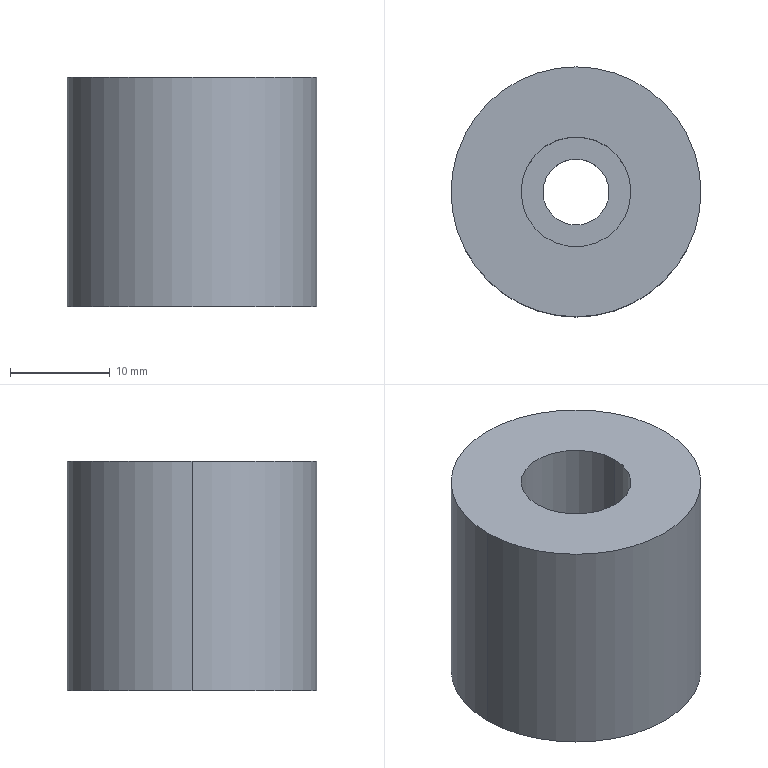Part | SolidWorks | features Extrusion 1, HoleWzd 1 | 1 solid | 9 faces | box 25 x 25 x 23 mm | volume 9481 mm3 | cylinder 6 | plane 3 | commonest cylinder face diameters 6.6 x2 11 x2 25 x2
STEP:
#1=CARTESIAN_POINT('',(-5.5,0.,6.2));
#2=VERTEX_POINT('',#1);
#3=CARTESIAN_POINT('',(5.5,0.,6.2));
#4=VERTEX_POINT('',#3);
#5=CARTESIAN_POINT('',(0.,0.,6.2));
#6=DIRECTION('',(0.,0.,1.));
#7=DIRECTION('',(1.,0.,0.));
#8=AXIS2_PLACEMENT_3D('',#5,#6,#7);
#9=CIRCLE('',#8,5.5);
#10=EDGE_CURVE('',#2,#4,#9,.T.);
#11=ORIENTED_EDGE('',*,*,#10,.F.);
#12=CARTESIAN_POINT('',(-5.5,0.,23.));
#13=VERTEX_POINT('',#12);
#14=CARTESIAN_POINT('',(-5.5,0.,23.));
#15=DIRECTION('',(0.,0.,1.));
#16=VECTOR('',#15,1000.);
#17=LINE('',#14,#16);
#18=EDGE_CURVE('',#2,#13,#17,.T.);
#19=ORIENTED_EDGE('',*,*,#18,.T.);
#20=CARTESIAN_POINT('',(5.5,0.,23.));
#21=VERTEX_POINT('',#20);
#22=CARTESIAN_POINT('',(0.,0.,23.));
#23=DIRECTION('',(0.,0.,1.));
#24=DIRECTION('',(1.,0.,0.));
#25=AXIS2_PLACEMENT_3D('',#22,#23,#24);
#26=CIRCLE('',#25,5.5);
#27=EDGE_CURVE('',#13,#21,#26,.T.);
#28=ORIENTED_EDGE('',*,*,#27,.T.);
#29=CARTESIAN_POINT('',(5.5,0.,23.));
#30=DIRECTION('',(0.,0.,1.));
#31=VECTOR('',#30,1000.);
#32=LINE('',#29,#31);
#33=EDGE_CURVE('',#4,#21,#32,.T.);
#34=ORIENTED_EDGE('',*,*,#33,.F.);
#35=EDGE_LOOP('',(#11,#19,#28,#34));
#36=FACE_OUTER_BOUND('',#35,.T.);
#37=CARTESIAN_POINT('',(0.,0.,23.));
#38=DIRECTION('',(0.,0.,1.));
#39=DIRECTION('',(1.,0.,0.));
#40=AXIS2_PLACEMENT_3D('',#37,#38,#39);
#41=CYLINDRICAL_SURFACE('',#40,5.5);
#42=ADVANCED_FACE('',(#36),#41,.F.);
#43=CARTESIAN_POINT('',(-3.3,0.,0.));
#44=VERTEX_POINT('',#43);
#45=CARTESIAN_POINT('',(3.3,0.,0.));
#46=VERTEX_POINT('',#45);
#47=CARTESIAN_POINT('',(0.,0.,0.));
#48=DIRECTION('',(0.,0.,1.));
#49=DIRECTION('',(1.,0.,0.));
#50=AXIS2_PLACEMENT_3D('',#47,#48,#49);
#51=CIRCLE('',#50,3.3);
#52=EDGE_CURVE('',#44,#46,#51,.T.);
#53=ORIENTED_EDGE('',*,*,#52,.F.);
#54=CARTESIAN_POINT('',(-3.3,0.,6.2));
#55=VERTEX_POINT('',#54);
#56=CARTESIAN_POINT('',(-3.3,0.,23.));
#57=DIRECTION('',(0.,0.,1.));
#58=VECTOR('',#57,1000.);
#59=LINE('',#56,#58);
#60=EDGE_CURVE('',#44,#55,#59,.T.);
#61=ORIENTED_EDGE('',*,*,#60,.T.);
#62=CARTESIAN_POINT('',(3.3,0.,6.2));
#63=VERTEX_POINT('',#62);
#64=CARTESIAN_POINT('',(0.,0.,6.2));
#65=DIRECTION('',(0.,0.,1.));
#66=DIRECTION('',(1.,0.,0.));
#67=AXIS2_PLACEMENT_3D('',#64,#65,#66);
#68=CIRCLE('',#67,3.3);
#69=EDGE_CURVE('',#55,#63,#68,.T.);
#70=ORIENTED_EDGE('',*,*,#69,.T.);
#71=CARTESIAN_POINT('',(3.3,0.,23.));
#72=DIRECTION('',(0.,0.,1.));
#73=VECTOR('',#72,1000.);
#74=LINE('',#71,#73);
#75=EDGE_CURVE('',#46,#63,#74,.T.);
#76=ORIENTED_EDGE('',*,*,#75,.F.);
#77=EDGE_LOOP('',(#53,#61,#70,#76));
#78=FACE_OUTER_BOUND('',#77,.T.);
#79=CARTESIAN_POINT('',(0.,0.,23.));
#80=DIRECTION('',(0.,0.,1.));
#81=DIRECTION('',(1.,0.,0.));
#82=AXIS2_PLACEMENT_3D('',#79,#80,#81);
#83=CYLINDRICAL_SURFACE('',#82,3.3);
#84=ADVANCED_FACE('',(#78),#83,.F.);
#85=CARTESIAN_POINT('',(12.5,0.,23.));
#86=VERTEX_POINT('',#85);
#87=CARTESIAN_POINT('',(-12.5,0.,23.));
#88=VERTEX_POINT('',#87);
#89=CARTESIAN_POINT('',(0.,0.,23.));
#90=DIRECTION('',(0.,0.,1.));
#91=DIRECTION('',(1.,0.,0.));
#92=AXIS2_PLACEMENT_3D('',#89,#90,#91);
#93=CIRCLE('',#92,12.5);
#94=EDGE_CURVE('',#86,#88,#93,.T.);
#95=ORIENTED_EDGE('',*,*,#94,.F.);
#96=CARTESIAN_POINT('',(12.5,0.,0.));
#97=VERTEX_POINT('',#96);
#98=CARTESIAN_POINT('',(12.5,0.,23.));
#99=DIRECTION('',(0.,0.,-1.));
#100=VECTOR('',#99,1000.);
#101=LINE('',#98,#100);
#102=EDGE_CURVE('',#86,#97,#101,.T.);
#103=ORIENTED_EDGE('',*,*,#102,.T.);
#104=CARTESIAN_POINT('',(-12.5,0.,0.));
#105=VERTEX_POINT('',#104);
#106=CARTESIAN_POINT('',(0.,0.,0.));
#107=DIRECTION('',(0.,0.,1.));
#108=DIRECTION('',(1.,0.,0.));
#109=AXIS2_PLACEMENT_3D('',#106,#107,#108);
#110=CIRCLE('',#109,12.5);
#111=EDGE_CURVE('',#97,#105,#110,.T.);
#112=ORIENTED_EDGE('',*,*,#111,.T.);
#113=CARTESIAN_POINT('',(-12.5,0.,23.));
#114=DIRECTION('',(0.,0.,-1.));
#115=VECTOR('',#114,1000.);
#116=LINE('',#113,#115);
#117=EDGE_CURVE('',#88,#105,#116,.T.);
#118=ORIENTED_EDGE('',*,*,#117,.F.);
#119=EDGE_LOOP('',(#95,#103,#112,#118));
#120=FACE_OUTER_BOUND('',#119,.T.);
#121=CARTESIAN_POINT('',(0.,0.,23.));
#122=DIRECTION('',(0.,0.,-1.));
#123=DIRECTION('',(-1.,0.,0.));
#124=AXIS2_PLACEMENT_3D('',#121,#122,#123);
#125=CYLINDRICAL_SURFACE('',#124,12.5);
#126=ADVANCED_FACE('',(#120),#125,.T.);
#127=ORIENTED_EDGE('',*,*,#102,.F.);
#128=CARTESIAN_POINT('',(0.,0.,23.));
#129=DIRECTION('',(0.,0.,1.));
#130=DIRECTION('',(1.,0.,0.));
#131=AXIS2_PLACEMENT_3D('',#128,#129,#130);
#132=CIRCLE('',#131,12.5);
#133=EDGE_CURVE('',#88,#86,#132,.T.);
#134=ORIENTED_EDGE('',*,*,#133,.F.);
#135=ORIENTED_EDGE('',*,*,#117,.T.);
#136=CARTESIAN_POINT('',(0.,0.,0.));
#137=DIRECTION('',(0.,0.,1.));
#138=DIRECTION('',(1.,0.,0.));
#139=AXIS2_PLACEMENT_3D('',#136,#137,#138);
#140=CIRCLE('',#139,12.5);
#141=EDGE_CURVE('',#105,#97,#140,.T.);
#142=ORIENTED_EDGE('',*,*,#141,.T.);
#143=EDGE_LOOP('',(#127,#134,#135,#142));
#144=FACE_OUTER_BOUND('',#143,.T.);
#145=CARTESIAN_POINT('',(0.,0.,23.));
#146=DIRECTION('',(0.,0.,-1.));
#147=DIRECTION('',(-1.,0.,0.));
#148=AXIS2_PLACEMENT_3D('',#145,#146,#147);
#149=CYLINDRICAL_SURFACE('',#148,12.5);
#150=ADVANCED_FACE('',(#144),#149,.T.);
#151=CARTESIAN_POINT('',(0.,0.,23.));
#152=DIRECTION('',(0.,0.,1.));
#153=DIRECTION('',(1.,0.,0.));
#154=AXIS2_PLACEMENT_3D('',#151,#152,#153);
#155=CIRCLE('',#154,5.5);
#156=EDGE_CURVE('',#21,#13,#155,.T.);
#157=ORIENTED_EDGE('',*,*,#156,.F.);
#158=ORIENTED_EDGE('',*,*,#27,.F.);
#159=EDGE_LOOP('',(#157,#158));
#160=FACE_BOUND('',#159,.T.);
#161=ORIENTED_EDGE('',*,*,#133,.T.);
#162=ORIENTED_EDGE('',*,*,#94,.T.);
#163=EDGE_LOOP('',(#161,#162));
#164=FACE_OUTER_BOUND('',#163,.T.);
#165=CARTESIAN_POINT('',(0.,0.,23.));
#166=DIRECTION('',(0.,0.,1.));
#167=DIRECTION('',(1.,0.,0.));
#168=AXIS2_PLACEMENT_3D('',#165,#166,#167);
#169=PLANE('',#168);
#170=ADVANCED_FACE('',(#160,#164),#169,.T.);
#171=CARTESIAN_POINT('',(0.,0.,0.));
#172=DIRECTION('',(0.,0.,1.));
#173=DIRECTION('',(1.,0.,0.));
#174=AXIS2_PLACEMENT_3D('',#171,#172,#173);
#175=CIRCLE('',#174,3.3);
#176=EDGE_CURVE('',#46,#44,#175,.T.);
#177=ORIENTED_EDGE('',*,*,#176,.T.);
#178=ORIENTED_EDGE('',*,*,#52,.T.);
#179=EDGE_LOOP('',(#177,#178));
#180=FACE_BOUND('',#179,.T.);
#181=ORIENTED_EDGE('',*,*,#141,.F.);
#182=ORIENTED_EDGE('',*,*,#111,.F.);
#183=EDGE_LOOP('',(#181,#182));
#184=FACE_OUTER_BOUND('',#183,.T.);
#185=CARTESIAN_POINT('',(0.,0.,0.));
#186=DIRECTION('',(0.,0.,1.));
#187=DIRECTION('',(1.,0.,0.));
#188=AXIS2_PLACEMENT_3D('',#185,#186,#187);
#189=PLANE('',#188);
#190=ADVANCED_FACE('',(#180,#184),#189,.F.);
#191=ORIENTED_EDGE('',*,*,#60,.F.);
#192=ORIENTED_EDGE('',*,*,#176,.F.);
#193=ORIENTED_EDGE('',*,*,#75,.T.);
#194=CARTESIAN_POINT('',(0.,0.,6.2));
#195=DIRECTION('',(0.,0.,1.));
#196=DIRECTION('',(1.,0.,0.));
#197=AXIS2_PLACEMENT_3D('',#194,#195,#196);
#198=CIRCLE('',#197,3.3);
#199=EDGE_CURVE('',#63,#55,#198,.T.);
#200=ORIENTED_EDGE('',*,*,#199,.T.);
#201=EDGE_LOOP('',(#191,#192,#193,#200));
#202=FACE_OUTER_BOUND('',#201,.T.);
#203=CARTESIAN_POINT('',(0.,0.,23.));
#204=DIRECTION('',(0.,0.,1.));
#205=DIRECTION('',(1.,0.,0.));
#206=AXIS2_PLACEMENT_3D('',#203,#204,#205);
#207=CYLINDRICAL_SURFACE('',#206,3.3);
#208=ADVANCED_FACE('',(#202),#207,.F.);
#209=ORIENTED_EDGE('',*,*,#199,.F.);
#210=ORIENTED_EDGE('',*,*,#69,.F.);
#211=EDGE_LOOP('',(#209,#210));
#212=FACE_BOUND('',#211,.T.);
#213=CARTESIAN_POINT('',(0.,0.,6.2));
#214=DIRECTION('',(0.,0.,1.));
#215=DIRECTION('',(1.,0.,0.));
#216=AXIS2_PLACEMENT_3D('',#213,#214,#215);
#217=CIRCLE('',#216,5.5);
#218=EDGE_CURVE('',#4,#2,#217,.T.);
#219=ORIENTED_EDGE('',*,*,#218,.T.);
#220=ORIENTED_EDGE('',*,*,#10,.T.);
#221=EDGE_LOOP('',(#219,#220));
#222=FACE_OUTER_BOUND('',#221,.T.);
#223=CARTESIAN_POINT('',(3.3,0.,6.2));
#224=DIRECTION('',(0.,0.,-1.));
#225=DIRECTION('',(-1.,0.,0.));
#226=AXIS2_PLACEMENT_3D('',#223,#224,#225);
#227=PLANE('',#226);
#228=ADVANCED_FACE('',(#212,#222),#227,.F.);
#229=ORIENTED_EDGE('',*,*,#18,.F.);
#230=ORIENTED_EDGE('',*,*,#218,.F.);
#231=ORIENTED_EDGE('',*,*,#33,.T.);
#232=ORIENTED_EDGE('',*,*,#156,.T.);
#233=EDGE_LOOP('',(#229,#230,#231,#232));
#234=FACE_OUTER_BOUND('',#233,.T.);
#235=CARTESIAN_POINT('',(0.,0.,23.));
#236=DIRECTION('',(0.,0.,1.));
#237=DIRECTION('',(1.,0.,0.));
#238=AXIS2_PLACEMENT_3D('',#235,#236,#237);
#239=CYLINDRICAL_SURFACE('',#238,5.5);
#240=ADVANCED_FACE('',(#234),#239,.F.);
#241=CLOSED_SHELL('',(#42,#84,#126,#150,#170,#190,#208,#228,#240));
#242=MANIFOLD_SOLID_BREP('',#241);
#243=CARTESIAN_POINT('',(0.,0.,0.));
#244=DIRECTION('',(0.,0.,1.));
#245=DIRECTION('',(1.,0.,0.));
#246=AXIS2_PLACEMENT_3D('',#243,#244,#245);
#247=(LENGTH_UNIT()NAMED_UNIT(*)SI_UNIT(.MILLI.,.METRE.));
#248=UNCERTAINTY_MEASURE_WITH_UNIT(LENGTH_MEASURE(0.00001),#247,'','');
#249=(NAMED_UNIT(*)PLANE_ANGLE_UNIT()SI_UNIT($,.RADIAN.));
#250=(NAMED_UNIT(*)SI_UNIT($,.STERADIAN.)SOLID_ANGLE_UNIT());
#251=(GEOMETRIC_REPRESENTATION_CONTEXT(3)GLOBAL_UNCERTAINTY_ASSIGNED_CONTEXT((#248))GLOBAL_UNIT_ASSIGNED_CONTEXT((#247,#249,#250))REPRESENTATION_CONTEXT('',''));
#252=ADVANCED_BREP_SHAPE_REPRESENTATION('',(#242,#246),#251);